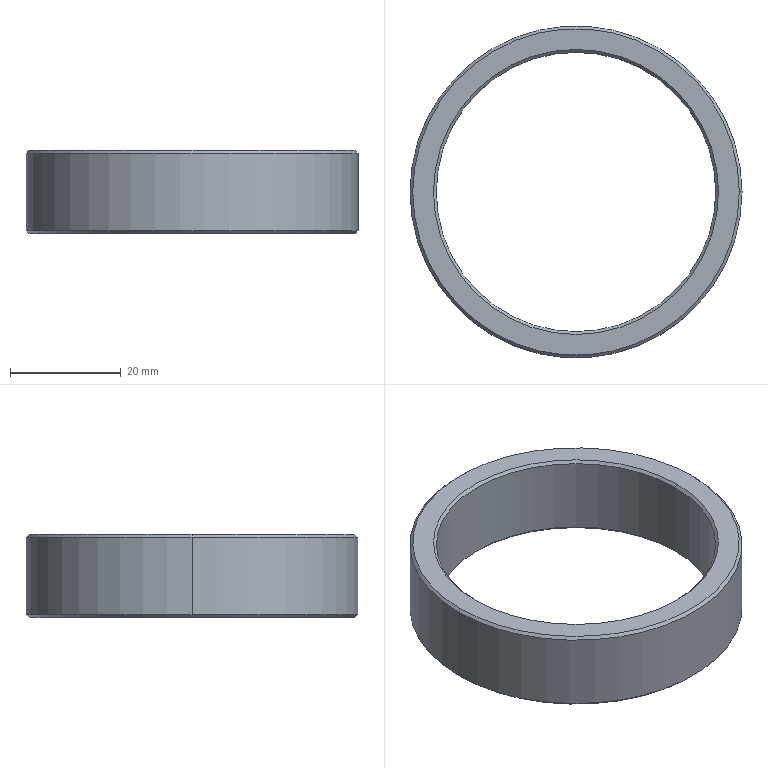Part | SolidWorks | features BaseBody 1 | 1 solid | 14 faces | box 60 x 60 x 15 mm | volume 12280 mm3 | cone 8 | cylinder 4 | plane 2 | commonest cylinder face diameters 50.5 x2 60 x2
STEP:
#1=CARTESIAN_POINT('',(-25.25,0.,7.));
#2=VERTEX_POINT('',#1);
#3=CARTESIAN_POINT('',(25.25,0.,7.));
#4=VERTEX_POINT('',#3);
#5=CARTESIAN_POINT('',(0.,0.,7.));
#6=DIRECTION('',(0.,0.,1.));
#7=DIRECTION('',(1.,0.,0.));
#8=AXIS2_PLACEMENT_3D('',#5,#6,#7);
#9=CIRCLE('',#8,25.25);
#10=EDGE_CURVE('',#2,#4,#9,.T.);
#11=ORIENTED_EDGE('',*,*,#10,.F.);
#12=CARTESIAN_POINT('',(-25.75,0.,7.5));
#13=VERTEX_POINT('',#12);
#14=CARTESIAN_POINT('',(-25.25,0.,7.));
#15=DIRECTION('',(-0.7071,0.,0.7071));
#16=VECTOR('',#15,1000.);
#17=LINE('',#14,#16);
#18=EDGE_CURVE('',#2,#13,#17,.T.);
#19=ORIENTED_EDGE('',*,*,#18,.T.);
#20=CARTESIAN_POINT('',(25.75,0.,7.5));
#21=VERTEX_POINT('',#20);
#22=CARTESIAN_POINT('',(0.,0.,7.5));
#23=DIRECTION('',(0.,0.,-1.));
#24=DIRECTION('',(1.,0.,0.));
#25=AXIS2_PLACEMENT_3D('',#22,#23,#24);
#26=CIRCLE('',#25,25.75);
#27=EDGE_CURVE('',#21,#13,#26,.T.);
#28=ORIENTED_EDGE('',*,*,#27,.F.);
#29=CARTESIAN_POINT('',(25.25,0.,7.));
#30=DIRECTION('',(0.7071,0.,0.7071));
#31=VECTOR('',#30,1000.);
#32=LINE('',#29,#31);
#33=EDGE_CURVE('',#4,#21,#32,.T.);
#34=ORIENTED_EDGE('',*,*,#33,.F.);
#35=EDGE_LOOP('',(#11,#19,#28,#34));
#36=FACE_OUTER_BOUND('',#35,.T.);
#37=CARTESIAN_POINT('',(0.,0.,7.));
#38=DIRECTION('',(0.,0.,1.));
#39=DIRECTION('',(1.,0.,0.));
#40=AXIS2_PLACEMENT_3D('',#37,#38,#39);
#41=CONICAL_SURFACE('',#40,25.25,0.7854);
#42=ADVANCED_FACE('',(#36),#41,.F.);
#43=CARTESIAN_POINT('',(29.5,0.,7.5));
#44=VERTEX_POINT('',#43);
#45=CARTESIAN_POINT('',(-29.5,0.,7.5));
#46=VERTEX_POINT('',#45);
#47=CARTESIAN_POINT('',(0.,0.,7.5));
#48=DIRECTION('',(0.,0.,1.));
#49=DIRECTION('',(1.,0.,0.));
#50=AXIS2_PLACEMENT_3D('',#47,#48,#49);
#51=CIRCLE('',#50,29.5);
#52=EDGE_CURVE('',#44,#46,#51,.T.);
#53=ORIENTED_EDGE('',*,*,#52,.F.);
#54=CARTESIAN_POINT('',(30.,0.,7.));
#55=VERTEX_POINT('',#54);
#56=CARTESIAN_POINT('',(29.5,0.,7.5));
#57=DIRECTION('',(0.7071,0.,-0.7071));
#58=VECTOR('',#57,1000.);
#59=LINE('',#56,#58);
#60=EDGE_CURVE('',#44,#55,#59,.T.);
#61=ORIENTED_EDGE('',*,*,#60,.T.);
#62=CARTESIAN_POINT('',(-30.,0.,7.));
#63=VERTEX_POINT('',#62);
#64=CARTESIAN_POINT('',(0.,0.,7.));
#65=DIRECTION('',(0.,0.,-1.));
#66=DIRECTION('',(1.,0.,0.));
#67=AXIS2_PLACEMENT_3D('',#64,#65,#66);
#68=CIRCLE('',#67,30.);
#69=EDGE_CURVE('',#63,#55,#68,.T.);
#70=ORIENTED_EDGE('',*,*,#69,.F.);
#71=CARTESIAN_POINT('',(-29.5,0.,7.5));
#72=DIRECTION('',(-0.7071,0.,-0.7071));
#73=VECTOR('',#72,1000.);
#74=LINE('',#71,#73);
#75=EDGE_CURVE('',#46,#63,#74,.T.);
#76=ORIENTED_EDGE('',*,*,#75,.F.);
#77=EDGE_LOOP('',(#53,#61,#70,#76));
#78=FACE_OUTER_BOUND('',#77,.T.);
#79=CARTESIAN_POINT('',(0.,0.,7.5));
#80=DIRECTION('',(0.,0.,-1.));
#81=DIRECTION('',(-1.,0.,0.));
#82=AXIS2_PLACEMENT_3D('',#79,#80,#81);
#83=CONICAL_SURFACE('',#82,29.5,0.7854);
#84=ADVANCED_FACE('',(#78),#83,.T.);
#85=CARTESIAN_POINT('',(25.25,0.,-7.));
#86=VERTEX_POINT('',#85);
#87=CARTESIAN_POINT('',(-25.25,0.,-7.));
#88=VERTEX_POINT('',#87);
#89=CARTESIAN_POINT('',(0.,0.,-7.));
#90=DIRECTION('',(0.,0.,-1.));
#91=DIRECTION('',(1.,0.,0.));
#92=AXIS2_PLACEMENT_3D('',#89,#90,#91);
#93=CIRCLE('',#92,25.25);
#94=EDGE_CURVE('',#86,#88,#93,.T.);
#95=ORIENTED_EDGE('',*,*,#94,.F.);
#96=CARTESIAN_POINT('',(25.75,0.,-7.5));
#97=VERTEX_POINT('',#96);
#98=CARTESIAN_POINT('',(25.75,0.,-7.5));
#99=DIRECTION('',(0.7071,0.,-0.7071));
#100=VECTOR('',#99,1000.);
#101=LINE('',#98,#100);
#102=EDGE_CURVE('',#86,#97,#101,.T.);
#103=ORIENTED_EDGE('',*,*,#102,.T.);
#104=CARTESIAN_POINT('',(-25.75,0.,-7.5));
#105=VERTEX_POINT('',#104);
#106=CARTESIAN_POINT('',(0.,0.,-7.5));
#107=DIRECTION('',(0.,0.,1.));
#108=DIRECTION('',(1.,0.,0.));
#109=AXIS2_PLACEMENT_3D('',#106,#107,#108);
#110=CIRCLE('',#109,25.75);
#111=EDGE_CURVE('',#105,#97,#110,.T.);
#112=ORIENTED_EDGE('',*,*,#111,.F.);
#113=CARTESIAN_POINT('',(-25.75,0.,-7.5));
#114=DIRECTION('',(-0.7071,0.,-0.7071));
#115=VECTOR('',#114,1000.);
#116=LINE('',#113,#115);
#117=EDGE_CURVE('',#88,#105,#116,.T.);
#118=ORIENTED_EDGE('',*,*,#117,.F.);
#119=EDGE_LOOP('',(#95,#103,#112,#118));
#120=FACE_OUTER_BOUND('',#119,.T.);
#121=CARTESIAN_POINT('',(0.,0.,-7.5));
#122=DIRECTION('',(0.,0.,-1.));
#123=DIRECTION('',(-1.,0.,0.));
#124=AXIS2_PLACEMENT_3D('',#121,#122,#123);
#125=CONICAL_SURFACE('',#124,25.75,0.7854);
#126=ADVANCED_FACE('',(#120),#125,.F.);
#127=CARTESIAN_POINT('',(-29.5,0.,-7.5));
#128=VERTEX_POINT('',#127);
#129=CARTESIAN_POINT('',(29.5,0.,-7.5));
#130=VERTEX_POINT('',#129);
#131=CARTESIAN_POINT('',(0.,0.,-7.5));
#132=DIRECTION('',(0.,0.,-1.));
#133=DIRECTION('',(1.,0.,0.));
#134=AXIS2_PLACEMENT_3D('',#131,#132,#133);
#135=CIRCLE('',#134,29.5);
#136=EDGE_CURVE('',#128,#130,#135,.T.);
#137=ORIENTED_EDGE('',*,*,#136,.F.);
#138=CARTESIAN_POINT('',(-30.,0.,-7.));
#139=VERTEX_POINT('',#138);
#140=CARTESIAN_POINT('',(-30.,0.,-7.));
#141=DIRECTION('',(-0.7071,0.,0.7071));
#142=VECTOR('',#141,1000.);
#143=LINE('',#140,#142);
#144=EDGE_CURVE('',#128,#139,#143,.T.);
#145=ORIENTED_EDGE('',*,*,#144,.T.);
#146=CARTESIAN_POINT('',(30.,0.,-7.));
#147=VERTEX_POINT('',#146);
#148=CARTESIAN_POINT('',(0.,0.,-7.));
#149=DIRECTION('',(0.,0.,1.));
#150=DIRECTION('',(1.,0.,0.));
#151=AXIS2_PLACEMENT_3D('',#148,#149,#150);
#152=CIRCLE('',#151,30.);
#153=EDGE_CURVE('',#147,#139,#152,.T.);
#154=ORIENTED_EDGE('',*,*,#153,.F.);
#155=CARTESIAN_POINT('',(30.,0.,-7.));
#156=DIRECTION('',(0.7071,0.,0.7071));
#157=VECTOR('',#156,1000.);
#158=LINE('',#155,#157);
#159=EDGE_CURVE('',#130,#147,#158,.T.);
#160=ORIENTED_EDGE('',*,*,#159,.F.);
#161=EDGE_LOOP('',(#137,#145,#154,#160));
#162=FACE_OUTER_BOUND('',#161,.T.);
#163=CARTESIAN_POINT('',(0.,0.,-7.));
#164=DIRECTION('',(0.,0.,1.));
#165=DIRECTION('',(1.,0.,0.));
#166=AXIS2_PLACEMENT_3D('',#163,#164,#165);
#167=CONICAL_SURFACE('',#166,30.,0.7854);
#168=ADVANCED_FACE('',(#162),#167,.T.);
#169=ORIENTED_EDGE('',*,*,#10,.T.);
#170=CARTESIAN_POINT('',(25.25,0.,7.5));
#171=DIRECTION('',(0.,0.,-1.));
#172=VECTOR('',#171,1000.);
#173=LINE('',#170,#172);
#174=EDGE_CURVE('',#4,#86,#173,.T.);
#175=ORIENTED_EDGE('',*,*,#174,.T.);
#176=ORIENTED_EDGE('',*,*,#94,.T.);
#177=CARTESIAN_POINT('',(-25.25,0.,7.5));
#178=DIRECTION('',(0.,0.,-1.));
#179=VECTOR('',#178,1000.);
#180=LINE('',#177,#179);
#181=EDGE_CURVE('',#2,#88,#180,.T.);
#182=ORIENTED_EDGE('',*,*,#181,.F.);
#183=EDGE_LOOP('',(#169,#175,#176,#182));
#184=FACE_OUTER_BOUND('',#183,.T.);
#185=CARTESIAN_POINT('',(0.,0.,7.5));
#186=DIRECTION('',(0.,0.,-1.));
#187=DIRECTION('',(-1.,0.,0.));
#188=AXIS2_PLACEMENT_3D('',#185,#186,#187);
#189=CYLINDRICAL_SURFACE('',#188,25.25);
#190=ADVANCED_FACE('',(#184),#189,.F.);
#191=ORIENTED_EDGE('',*,*,#69,.T.);
#192=CARTESIAN_POINT('',(30.,0.,7.5));
#193=DIRECTION('',(0.,0.,-1.));
#194=VECTOR('',#193,1000.);
#195=LINE('',#192,#194);
#196=EDGE_CURVE('',#55,#147,#195,.T.);
#197=ORIENTED_EDGE('',*,*,#196,.T.);
#198=ORIENTED_EDGE('',*,*,#153,.T.);
#199=CARTESIAN_POINT('',(-30.,0.,7.5));
#200=DIRECTION('',(0.,0.,-1.));
#201=VECTOR('',#200,1000.);
#202=LINE('',#199,#201);
#203=EDGE_CURVE('',#63,#139,#202,.T.);
#204=ORIENTED_EDGE('',*,*,#203,.F.);
#205=EDGE_LOOP('',(#191,#197,#198,#204));
#206=FACE_OUTER_BOUND('',#205,.T.);
#207=CARTESIAN_POINT('',(0.,0.,7.5));
#208=DIRECTION('',(0.,0.,-1.));
#209=DIRECTION('',(-1.,0.,0.));
#210=AXIS2_PLACEMENT_3D('',#207,#208,#209);
#211=CYLINDRICAL_SURFACE('',#210,30.);
#212=ADVANCED_FACE('',(#206),#211,.T.);
#213=CARTESIAN_POINT('',(0.,0.,7.5));
#214=DIRECTION('',(0.,0.,1.));
#215=DIRECTION('',(1.,0.,0.));
#216=AXIS2_PLACEMENT_3D('',#213,#214,#215);
#217=CIRCLE('',#216,29.5);
#218=EDGE_CURVE('',#46,#44,#217,.T.);
#219=ORIENTED_EDGE('',*,*,#218,.T.);
#220=ORIENTED_EDGE('',*,*,#52,.T.);
#221=EDGE_LOOP('',(#219,#220));
#222=FACE_OUTER_BOUND('',#221,.T.);
#223=ORIENTED_EDGE('',*,*,#27,.T.);
#224=CARTESIAN_POINT('',(0.,0.,7.5));
#225=DIRECTION('',(0.,0.,-1.));
#226=DIRECTION('',(1.,0.,0.));
#227=AXIS2_PLACEMENT_3D('',#224,#225,#226);
#228=CIRCLE('',#227,25.75);
#229=EDGE_CURVE('',#13,#21,#228,.T.);
#230=ORIENTED_EDGE('',*,*,#229,.T.);
#231=EDGE_LOOP('',(#223,#230));
#232=FACE_BOUND('',#231,.T.);
#233=CARTESIAN_POINT('',(0.,0.,7.5));
#234=DIRECTION('',(0.,0.,1.));
#235=DIRECTION('',(1.,0.,0.));
#236=AXIS2_PLACEMENT_3D('',#233,#234,#235);
#237=PLANE('',#236);
#238=ADVANCED_FACE('',(#222,#232),#237,.T.);
#239=CARTESIAN_POINT('',(0.,0.,-7.5));
#240=DIRECTION('',(0.,0.,-1.));
#241=DIRECTION('',(1.,0.,0.));
#242=AXIS2_PLACEMENT_3D('',#239,#240,#241);
#243=CIRCLE('',#242,29.5);
#244=EDGE_CURVE('',#130,#128,#243,.T.);
#245=ORIENTED_EDGE('',*,*,#244,.T.);
#246=ORIENTED_EDGE('',*,*,#136,.T.);
#247=EDGE_LOOP('',(#245,#246));
#248=FACE_OUTER_BOUND('',#247,.T.);
#249=ORIENTED_EDGE('',*,*,#111,.T.);
#250=CARTESIAN_POINT('',(0.,0.,-7.5));
#251=DIRECTION('',(0.,0.,1.));
#252=DIRECTION('',(1.,0.,0.));
#253=AXIS2_PLACEMENT_3D('',#250,#251,#252);
#254=CIRCLE('',#253,25.75);
#255=EDGE_CURVE('',#97,#105,#254,.T.);
#256=ORIENTED_EDGE('',*,*,#255,.T.);
#257=EDGE_LOOP('',(#249,#256));
#258=FACE_BOUND('',#257,.T.);
#259=CARTESIAN_POINT('',(0.,0.,-7.5));
#260=DIRECTION('',(0.,0.,1.));
#261=DIRECTION('',(1.,0.,0.));
#262=AXIS2_PLACEMENT_3D('',#259,#260,#261);
#263=PLANE('',#262);
#264=ADVANCED_FACE('',(#248,#258),#263,.F.);
#265=ORIENTED_EDGE('',*,*,#196,.F.);
#266=CARTESIAN_POINT('',(0.,0.,7.));
#267=DIRECTION('',(0.,0.,-1.));
#268=DIRECTION('',(1.,0.,0.));
#269=AXIS2_PLACEMENT_3D('',#266,#267,#268);
#270=CIRCLE('',#269,30.);
#271=EDGE_CURVE('',#55,#63,#270,.T.);
#272=ORIENTED_EDGE('',*,*,#271,.T.);
#273=ORIENTED_EDGE('',*,*,#203,.T.);
#274=CARTESIAN_POINT('',(0.,0.,-7.));
#275=DIRECTION('',(0.,0.,1.));
#276=DIRECTION('',(1.,0.,0.));
#277=AXIS2_PLACEMENT_3D('',#274,#275,#276);
#278=CIRCLE('',#277,30.);
#279=EDGE_CURVE('',#139,#147,#278,.T.);
#280=ORIENTED_EDGE('',*,*,#279,.T.);
#281=EDGE_LOOP('',(#265,#272,#273,#280));
#282=FACE_OUTER_BOUND('',#281,.T.);
#283=CARTESIAN_POINT('',(0.,0.,7.5));
#284=DIRECTION('',(0.,0.,-1.));
#285=DIRECTION('',(-1.,0.,0.));
#286=AXIS2_PLACEMENT_3D('',#283,#284,#285);
#287=CYLINDRICAL_SURFACE('',#286,30.);
#288=ADVANCED_FACE('',(#282),#287,.T.);
#289=ORIENTED_EDGE('',*,*,#174,.F.);
#290=CARTESIAN_POINT('',(0.,0.,7.));
#291=DIRECTION('',(0.,0.,1.));
#292=DIRECTION('',(1.,0.,0.));
#293=AXIS2_PLACEMENT_3D('',#290,#291,#292);
#294=CIRCLE('',#293,25.25);
#295=EDGE_CURVE('',#4,#2,#294,.T.);
#296=ORIENTED_EDGE('',*,*,#295,.T.);
#297=ORIENTED_EDGE('',*,*,#181,.T.);
#298=CARTESIAN_POINT('',(0.,0.,-7.));
#299=DIRECTION('',(0.,0.,-1.));
#300=DIRECTION('',(1.,0.,0.));
#301=AXIS2_PLACEMENT_3D('',#298,#299,#300);
#302=CIRCLE('',#301,25.25);
#303=EDGE_CURVE('',#88,#86,#302,.T.);
#304=ORIENTED_EDGE('',*,*,#303,.T.);
#305=EDGE_LOOP('',(#289,#296,#297,#304));
#306=FACE_OUTER_BOUND('',#305,.T.);
#307=CARTESIAN_POINT('',(0.,0.,7.5));
#308=DIRECTION('',(0.,0.,-1.));
#309=DIRECTION('',(-1.,0.,0.));
#310=AXIS2_PLACEMENT_3D('',#307,#308,#309);
#311=CYLINDRICAL_SURFACE('',#310,25.25);
#312=ADVANCED_FACE('',(#306),#311,.F.);
#313=ORIENTED_EDGE('',*,*,#144,.F.);
#314=ORIENTED_EDGE('',*,*,#244,.F.);
#315=ORIENTED_EDGE('',*,*,#159,.T.);
#316=ORIENTED_EDGE('',*,*,#279,.F.);
#317=EDGE_LOOP('',(#313,#314,#315,#316));
#318=FACE_OUTER_BOUND('',#317,.T.);
#319=CARTESIAN_POINT('',(0.,0.,-7.));
#320=DIRECTION('',(0.,0.,1.));
#321=DIRECTION('',(1.,0.,0.));
#322=AXIS2_PLACEMENT_3D('',#319,#320,#321);
#323=CONICAL_SURFACE('',#322,30.,0.7854);
#324=ADVANCED_FACE('',(#318),#323,.T.);
#325=ORIENTED_EDGE('',*,*,#102,.F.);
#326=ORIENTED_EDGE('',*,*,#303,.F.);
#327=ORIENTED_EDGE('',*,*,#117,.T.);
#328=ORIENTED_EDGE('',*,*,#255,.F.);
#329=EDGE_LOOP('',(#325,#326,#327,#328));
#330=FACE_OUTER_BOUND('',#329,.T.);
#331=CARTESIAN_POINT('',(0.,0.,-7.5));
#332=DIRECTION('',(0.,0.,-1.));
#333=DIRECTION('',(-1.,0.,0.));
#334=AXIS2_PLACEMENT_3D('',#331,#332,#333);
#335=CONICAL_SURFACE('',#334,25.75,0.7854);
#336=ADVANCED_FACE('',(#330),#335,.F.);
#337=ORIENTED_EDGE('',*,*,#60,.F.);
#338=ORIENTED_EDGE('',*,*,#218,.F.);
#339=ORIENTED_EDGE('',*,*,#75,.T.);
#340=ORIENTED_EDGE('',*,*,#271,.F.);
#341=EDGE_LOOP('',(#337,#338,#339,#340));
#342=FACE_OUTER_BOUND('',#341,.T.);
#343=CARTESIAN_POINT('',(0.,0.,7.5));
#344=DIRECTION('',(0.,0.,-1.));
#345=DIRECTION('',(-1.,0.,0.));
#346=AXIS2_PLACEMENT_3D('',#343,#344,#345);
#347=CONICAL_SURFACE('',#346,29.5,0.7854);
#348=ADVANCED_FACE('',(#342),#347,.T.);
#349=ORIENTED_EDGE('',*,*,#18,.F.);
#350=ORIENTED_EDGE('',*,*,#295,.F.);
#351=ORIENTED_EDGE('',*,*,#33,.T.);
#352=ORIENTED_EDGE('',*,*,#229,.F.);
#353=EDGE_LOOP('',(#349,#350,#351,#352));
#354=FACE_OUTER_BOUND('',#353,.T.);
#355=CARTESIAN_POINT('',(0.,0.,7.));
#356=DIRECTION('',(0.,0.,1.));
#357=DIRECTION('',(1.,0.,0.));
#358=AXIS2_PLACEMENT_3D('',#355,#356,#357);
#359=CONICAL_SURFACE('',#358,25.25,0.7854);
#360=ADVANCED_FACE('',(#354),#359,.F.);
#361=CLOSED_SHELL('',(#42,#84,#126,#168,#190,#212,#238,#264,#288,#312,#324,#336,#348,#360));
#362=MANIFOLD_SOLID_BREP('',#361);
#363=CARTESIAN_POINT('',(0.,0.,0.));
#364=DIRECTION('',(0.,0.,1.));
#365=DIRECTION('',(1.,0.,0.));
#366=AXIS2_PLACEMENT_3D('',#363,#364,#365);
#367=(LENGTH_UNIT()NAMED_UNIT(*)SI_UNIT(.MILLI.,.METRE.));
#368=UNCERTAINTY_MEASURE_WITH_UNIT(LENGTH_MEASURE(0.00001),#367,'','');
#369=(NAMED_UNIT(*)PLANE_ANGLE_UNIT()SI_UNIT($,.RADIAN.));
#370=(NAMED_UNIT(*)SI_UNIT($,.STERADIAN.)SOLID_ANGLE_UNIT());
#371=(GEOMETRIC_REPRESENTATION_CONTEXT(3)GLOBAL_UNCERTAINTY_ASSIGNED_CONTEXT((#368))GLOBAL_UNIT_ASSIGNED_CONTEXT((#367,#369,#370))REPRESENTATION_CONTEXT('',''));
#372=ADVANCED_BREP_SHAPE_REPRESENTATION('',(#362,#366),#371);